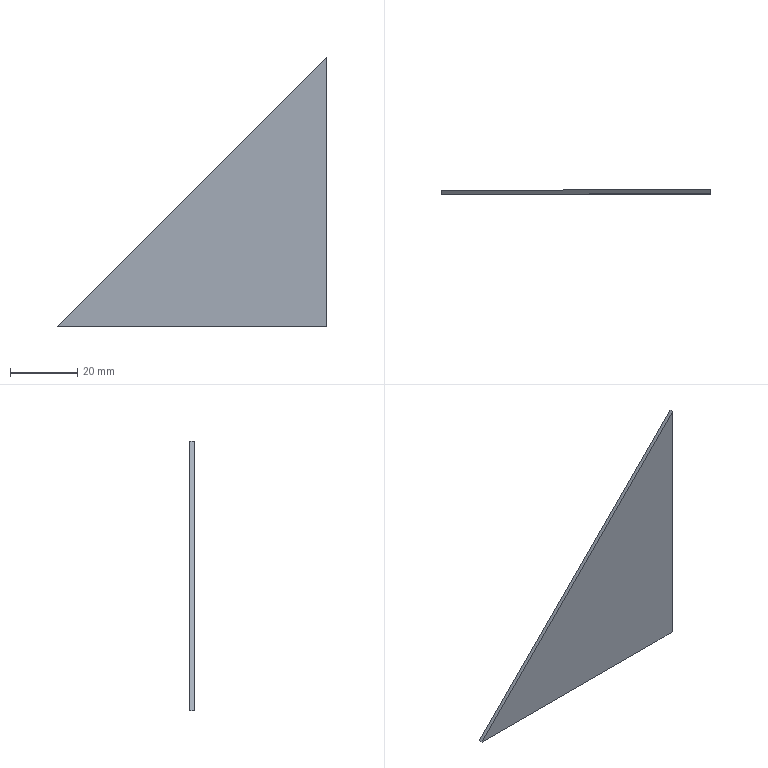Part | STEP file | 冲床-300配套压波_id378_x_t | 1 solid | 5 faces | box 80 x 1.2 x 80 mm | volume 3840 mm3 | plane 5
STEP:
#1=CARTESIAN_POINT('',(1428.,260.,-723.));
#2=VERTEX_POINT('',#1);
#3=CARTESIAN_POINT('',(1508.,260.,-723.));
#4=VERTEX_POINT('',#3);
#5=CARTESIAN_POINT('',(1428.,260.,-723.));
#6=DIRECTION('',(1.,0.,0.));
#7=VECTOR('',#6,1.);
#8=LINE('',#5,#7);
#9=EDGE_CURVE('',#2,#4,#8,.T.);
#10=ORIENTED_EDGE('',*,*,#9,.T.);
#11=CARTESIAN_POINT('',(1508.,258.8,-723.));
#12=VERTEX_POINT('',#11);
#13=CARTESIAN_POINT('',(1508.,258.8,-723.));
#14=DIRECTION('',(0.,1.,0.));
#15=VECTOR('',#14,1.);
#16=LINE('',#13,#15);
#17=EDGE_CURVE('',#12,#4,#16,.T.);
#18=ORIENTED_EDGE('',*,*,#17,.F.);
#19=CARTESIAN_POINT('',(1428.,258.8,-723.));
#20=VERTEX_POINT('',#19);
#21=CARTESIAN_POINT('',(1428.,258.8,-723.));
#22=DIRECTION('',(1.,0.,0.));
#23=VECTOR('',#22,1.);
#24=LINE('',#21,#23);
#25=EDGE_CURVE('',#20,#12,#24,.T.);
#26=ORIENTED_EDGE('',*,*,#25,.F.);
#27=CARTESIAN_POINT('',(1428.,258.8,-723.));
#28=DIRECTION('',(0.,1.,0.));
#29=VECTOR('',#28,1.);
#30=LINE('',#27,#29);
#31=EDGE_CURVE('',#20,#2,#30,.T.);
#32=ORIENTED_EDGE('',*,*,#31,.T.);
#33=EDGE_LOOP('',(#10,#18,#26,#32));
#34=FACE_OUTER_BOUND('',#33,.T.);
#35=CARTESIAN_POINT('',(1428.,258.8,-723.));
#36=DIRECTION('',(0.,0.,1.));
#37=DIRECTION('',(1.,0.,0.));
#38=AXIS2_PLACEMENT_3D('',#35,#36,#37);
#39=PLANE('',#38);
#40=ADVANCED_FACE('',(#34),#39,.F.);
#41=CARTESIAN_POINT('',(1508.,260.,-643.));
#42=VERTEX_POINT('',#41);
#43=CARTESIAN_POINT('',(1508.,260.,-723.));
#44=DIRECTION('',(0.,0.,1.));
#45=VECTOR('',#44,1.);
#46=LINE('',#43,#45);
#47=EDGE_CURVE('',#4,#42,#46,.T.);
#48=ORIENTED_EDGE('',*,*,#47,.T.);
#49=CARTESIAN_POINT('',(1508.,258.8,-643.));
#50=VERTEX_POINT('',#49);
#51=CARTESIAN_POINT('',(1508.,258.8,-643.));
#52=DIRECTION('',(0.,1.,0.));
#53=VECTOR('',#52,1.);
#54=LINE('',#51,#53);
#55=EDGE_CURVE('',#50,#42,#54,.T.);
#56=ORIENTED_EDGE('',*,*,#55,.F.);
#57=CARTESIAN_POINT('',(1508.,258.8,-723.));
#58=DIRECTION('',(0.,0.,1.));
#59=VECTOR('',#58,1.);
#60=LINE('',#57,#59);
#61=EDGE_CURVE('',#12,#50,#60,.T.);
#62=ORIENTED_EDGE('',*,*,#61,.F.);
#63=ORIENTED_EDGE('',*,*,#17,.T.);
#64=EDGE_LOOP('',(#48,#56,#62,#63));
#65=FACE_OUTER_BOUND('',#64,.T.);
#66=CARTESIAN_POINT('',(1508.,258.8,-723.));
#67=DIRECTION('',(-1.,0.,0.));
#68=DIRECTION('',(0.,0.,1.));
#69=AXIS2_PLACEMENT_3D('',#66,#67,#68);
#70=PLANE('',#69);
#71=ADVANCED_FACE('',(#65),#70,.F.);
#72=CARTESIAN_POINT('',(1508.,260.,-643.));
#73=DIRECTION('',(-0.7071,0.,-0.7071));
#74=VECTOR('',#73,1.);
#75=LINE('',#72,#74);
#76=EDGE_CURVE('',#42,#2,#75,.T.);
#77=ORIENTED_EDGE('',*,*,#76,.T.);
#78=ORIENTED_EDGE('',*,*,#31,.F.);
#79=CARTESIAN_POINT('',(1508.,258.8,-643.));
#80=DIRECTION('',(-0.7071,0.,-0.7071));
#81=VECTOR('',#80,1.);
#82=LINE('',#79,#81);
#83=EDGE_CURVE('',#50,#20,#82,.T.);
#84=ORIENTED_EDGE('',*,*,#83,.F.);
#85=ORIENTED_EDGE('',*,*,#55,.T.);
#86=EDGE_LOOP('',(#77,#78,#84,#85));
#87=FACE_OUTER_BOUND('',#86,.T.);
#88=CARTESIAN_POINT('',(1508.,258.8,-643.));
#89=DIRECTION('',(0.7071,0.,-0.7071));
#90=DIRECTION('',(-0.7071,0.,-0.7071));
#91=AXIS2_PLACEMENT_3D('',#88,#89,#90);
#92=PLANE('',#91);
#93=ADVANCED_FACE('',(#87),#92,.F.);
#94=ORIENTED_EDGE('',*,*,#25,.T.);
#95=ORIENTED_EDGE('',*,*,#61,.T.);
#96=ORIENTED_EDGE('',*,*,#83,.T.);
#97=EDGE_LOOP('',(#94,#95,#96));
#98=FACE_OUTER_BOUND('',#97,.T.);
#99=CARTESIAN_POINT('',(0.,258.8,0.));
#100=DIRECTION('',(0.,-1.,0.));
#101=DIRECTION('',(0.,0.,-1.));
#102=AXIS2_PLACEMENT_3D('',#99,#100,#101);
#103=PLANE('',#102);
#104=ADVANCED_FACE('',(#98),#103,.T.);
#105=ORIENTED_EDGE('',*,*,#9,.F.);
#106=ORIENTED_EDGE('',*,*,#76,.F.);
#107=ORIENTED_EDGE('',*,*,#47,.F.);
#108=EDGE_LOOP('',(#105,#106,#107));
#109=FACE_OUTER_BOUND('',#108,.T.);
#110=CARTESIAN_POINT('',(0.,260.,0.));
#111=DIRECTION('',(0.,-1.,0.));
#112=DIRECTION('',(0.,0.,-1.));
#113=AXIS2_PLACEMENT_3D('',#110,#111,#112);
#114=PLANE('',#113);
#115=ADVANCED_FACE('',(#109),#114,.F.);
#116=CLOSED_SHELL('',(#40,#71,#93,#104,#115));
#117=MANIFOLD_SOLID_BREP('',#116);
#118=(LENGTH_UNIT()NAMED_UNIT(*)SI_UNIT(.MILLI.,.METRE.));
#119=UNCERTAINTY_MEASURE_WITH_UNIT(LENGTH_MEASURE(0.00002),#118,'','');
#120=(NAMED_UNIT(*)PLANE_ANGLE_UNIT()SI_UNIT($,.RADIAN.));
#121=PLANE_ANGLE_MEASURE_WITH_UNIT(PLANE_ANGLE_MEASURE(0.01745),#120);
#122=DIMENSIONAL_EXPONENTS(0.,0.,0.,0.,0.,0.,0.);
#123=(CONVERSION_BASED_UNIT('DEGREE',#121)NAMED_UNIT(#122)PLANE_ANGLE_UNIT());
#124=(NAMED_UNIT(*)SI_UNIT($,.STERADIAN.)SOLID_ANGLE_UNIT());
#125=(GEOMETRIC_REPRESENTATION_CONTEXT(3)GLOBAL_UNCERTAINTY_ASSIGNED_CONTEXT((#119))GLOBAL_UNIT_ASSIGNED_CONTEXT((#118,#123,#124))REPRESENTATION_CONTEXT('',''));
#126=ADVANCED_BREP_SHAPE_REPRESENTATION('',(#117),#125);